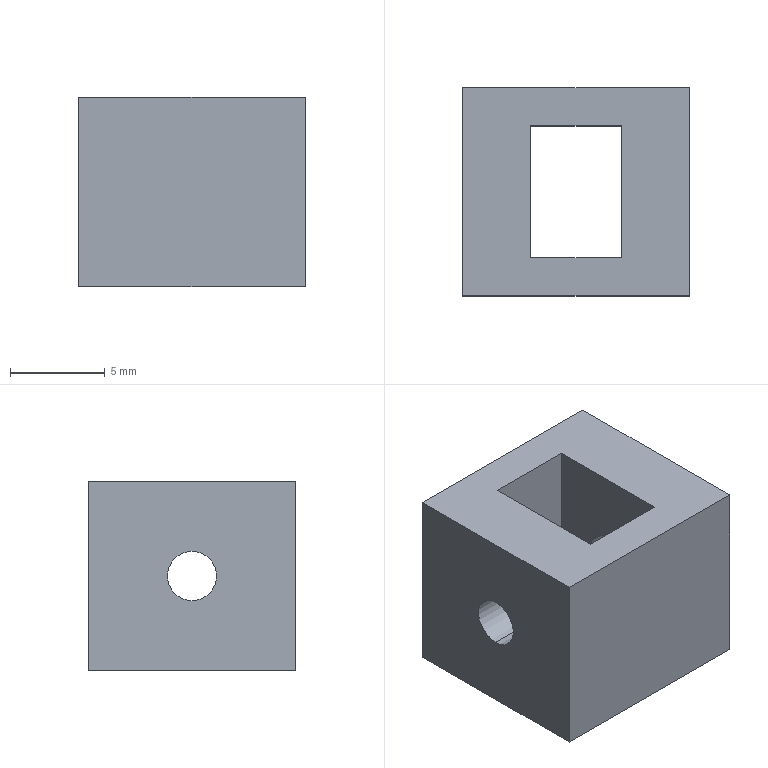Part | SolidWorks | features Extrusion 1, ICE 1 | 1 solid | 14 faces | box 11.98 x 10.98 x 10 mm | volume 942.243 mm3 | plane 10 | cylinder 4 | commonest cylinder face diameters 2.6 x4
STEP:
#1=CARTESIAN_POINT('',(-2.,3.49,6.3));
#2=VERTEX_POINT('',#1);
#3=CARTESIAN_POINT('',(-2.,3.49,3.7));
#4=VERTEX_POINT('',#3);
#5=CARTESIAN_POINT('',(-2.,3.49,5.));
#6=DIRECTION('',(1.,0.,0.));
#7=DIRECTION('',(0.,0.,-1.));
#8=AXIS2_PLACEMENT_3D('',#5,#6,#7);
#9=CIRCLE('',#8,1.3);
#10=EDGE_CURVE('',#2,#4,#9,.T.);
#11=ORIENTED_EDGE('',*,*,#10,.F.);
#12=CARTESIAN_POINT('',(1.59,3.49,6.3));
#13=VERTEX_POINT('',#12);
#14=CARTESIAN_POINT('',(-2.,3.49,6.3));
#15=DIRECTION('',(1.,0.,0.));
#16=VECTOR('',#15,1000.);
#17=LINE('',#14,#16);
#18=EDGE_CURVE('',#2,#13,#17,.T.);
#19=ORIENTED_EDGE('',*,*,#18,.T.);
#20=CARTESIAN_POINT('',(1.59,3.49,3.7));
#21=VERTEX_POINT('',#20);
#22=CARTESIAN_POINT('',(1.59,3.49,5.));
#23=DIRECTION('',(1.,0.,0.));
#24=DIRECTION('',(0.,1.,0.));
#25=AXIS2_PLACEMENT_3D('',#22,#23,#24);
#26=CIRCLE('',#25,1.3);
#27=EDGE_CURVE('',#13,#21,#26,.T.);
#28=ORIENTED_EDGE('',*,*,#27,.T.);
#29=CARTESIAN_POINT('',(-2.,3.49,3.7));
#30=DIRECTION('',(1.,0.,0.));
#31=VECTOR('',#30,1000.);
#32=LINE('',#29,#31);
#33=EDGE_CURVE('',#4,#21,#32,.T.);
#34=ORIENTED_EDGE('',*,*,#33,.F.);
#35=EDGE_LOOP('',(#11,#19,#28,#34));
#36=FACE_OUTER_BOUND('',#35,.T.);
#37=CARTESIAN_POINT('',(-2.,3.49,5.));
#38=DIRECTION('',(1.,0.,0.));
#39=DIRECTION('',(0.,0.,-1.));
#40=AXIS2_PLACEMENT_3D('',#37,#38,#39);
#41=CYLINDRICAL_SURFACE('',#40,1.3);
#42=ADVANCED_FACE('',(#36),#41,.F.);
#43=CARTESIAN_POINT('',(6.39,3.49,3.7));
#44=VERTEX_POINT('',#43);
#45=CARTESIAN_POINT('',(6.39,3.49,6.3));
#46=VERTEX_POINT('',#45);
#47=CARTESIAN_POINT('',(6.39,3.49,5.));
#48=DIRECTION('',(-1.,0.,0.));
#49=DIRECTION('',(0.,0.,1.));
#50=AXIS2_PLACEMENT_3D('',#47,#48,#49);
#51=CIRCLE('',#50,1.3);
#52=EDGE_CURVE('',#44,#46,#51,.T.);
#53=ORIENTED_EDGE('',*,*,#52,.T.);
#54=CARTESIAN_POINT('',(9.98,3.49,6.3));
#55=VERTEX_POINT('',#54);
#56=CARTESIAN_POINT('',(-2.,3.49,6.3));
#57=DIRECTION('',(1.,0.,0.));
#58=VECTOR('',#57,1000.);
#59=LINE('',#56,#58);
#60=EDGE_CURVE('',#46,#55,#59,.T.);
#61=ORIENTED_EDGE('',*,*,#60,.T.);
#62=CARTESIAN_POINT('',(9.98,3.49,3.7));
#63=VERTEX_POINT('',#62);
#64=CARTESIAN_POINT('',(9.98,3.49,5.));
#65=DIRECTION('',(1.,0.,0.));
#66=DIRECTION('',(0.,0.,-1.));
#67=AXIS2_PLACEMENT_3D('',#64,#65,#66);
#68=CIRCLE('',#67,1.3);
#69=EDGE_CURVE('',#55,#63,#68,.T.);
#70=ORIENTED_EDGE('',*,*,#69,.T.);
#71=CARTESIAN_POINT('',(-2.,3.49,3.7));
#72=DIRECTION('',(1.,0.,0.));
#73=VECTOR('',#72,1000.);
#74=LINE('',#71,#73);
#75=EDGE_CURVE('',#44,#63,#74,.T.);
#76=ORIENTED_EDGE('',*,*,#75,.F.);
#77=EDGE_LOOP('',(#53,#61,#70,#76));
#78=FACE_OUTER_BOUND('',#77,.T.);
#79=CARTESIAN_POINT('',(-2.,3.49,5.));
#80=DIRECTION('',(1.,0.,0.));
#81=DIRECTION('',(0.,0.,-1.));
#82=AXIS2_PLACEMENT_3D('',#79,#80,#81);
#83=CYLINDRICAL_SURFACE('',#82,1.3);
#84=ADVANCED_FACE('',(#78),#83,.F.);
#85=CARTESIAN_POINT('',(9.98,8.98,10.));
#86=VERTEX_POINT('',#85);
#87=CARTESIAN_POINT('',(-2.,8.98,10.));
#88=VERTEX_POINT('',#87);
#89=CARTESIAN_POINT('',(6.39,8.98,10.));
#90=DIRECTION('',(-1.,0.,0.));
#91=VECTOR('',#90,1000.);
#92=LINE('',#89,#91);
#93=EDGE_CURVE('',#86,#88,#92,.T.);
#94=ORIENTED_EDGE('',*,*,#93,.T.);
#95=CARTESIAN_POINT('',(-2.,-2.,10.));
#96=VERTEX_POINT('',#95);
#97=CARTESIAN_POINT('',(-2.,-2.,10.));
#98=DIRECTION('',(0.,-1.,0.));
#99=VECTOR('',#98,1000.);
#100=LINE('',#97,#99);
#101=EDGE_CURVE('',#88,#96,#100,.T.);
#102=ORIENTED_EDGE('',*,*,#101,.T.);
#103=CARTESIAN_POINT('',(9.98,-2.,10.));
#104=VERTEX_POINT('',#103);
#105=CARTESIAN_POINT('',(-2.,-2.,10.));
#106=DIRECTION('',(1.,0.,0.));
#107=VECTOR('',#106,1000.);
#108=LINE('',#105,#107);
#109=EDGE_CURVE('',#96,#104,#108,.T.);
#110=ORIENTED_EDGE('',*,*,#109,.T.);
#111=CARTESIAN_POINT('',(9.98,8.98,10.));
#112=DIRECTION('',(0.,1.,0.));
#113=VECTOR('',#112,1000.);
#114=LINE('',#111,#113);
#115=EDGE_CURVE('',#104,#86,#114,.T.);
#116=ORIENTED_EDGE('',*,*,#115,.T.);
#117=EDGE_LOOP('',(#94,#102,#110,#116));
#118=FACE_OUTER_BOUND('',#117,.T.);
#119=CARTESIAN_POINT('',(6.39,6.98,10.));
#120=VERTEX_POINT('',#119);
#121=CARTESIAN_POINT('',(1.59,6.98,10.));
#122=VERTEX_POINT('',#121);
#123=CARTESIAN_POINT('',(4.8,6.98,10.));
#124=DIRECTION('',(-1.,0.,0.));
#125=VECTOR('',#124,1000.);
#126=LINE('',#123,#125);
#127=EDGE_CURVE('',#120,#122,#126,.T.);
#128=ORIENTED_EDGE('',*,*,#127,.F.);
#129=CARTESIAN_POINT('',(6.39,0.,10.));
#130=VERTEX_POINT('',#129);
#131=CARTESIAN_POINT('',(6.39,6.98,10.));
#132=DIRECTION('',(0.,1.,0.));
#133=VECTOR('',#132,1000.);
#134=LINE('',#131,#133);
#135=EDGE_CURVE('',#130,#120,#134,.T.);
#136=ORIENTED_EDGE('',*,*,#135,.F.);
#137=CARTESIAN_POINT('',(1.59,0.,10.));
#138=VERTEX_POINT('',#137);
#139=CARTESIAN_POINT('',(1.59,0.,10.));
#140=DIRECTION('',(1.,0.,0.));
#141=VECTOR('',#140,1000.);
#142=LINE('',#139,#141);
#143=EDGE_CURVE('',#138,#130,#142,.T.);
#144=ORIENTED_EDGE('',*,*,#143,.F.);
#145=CARTESIAN_POINT('',(1.59,3.49,10.));
#146=DIRECTION('',(0.,-1.,0.));
#147=VECTOR('',#146,1000.);
#148=LINE('',#145,#147);
#149=EDGE_CURVE('',#122,#138,#148,.T.);
#150=ORIENTED_EDGE('',*,*,#149,.F.);
#151=EDGE_LOOP('',(#128,#136,#144,#150));
#152=FACE_BOUND('',#151,.T.);
#153=CARTESIAN_POINT('',(0.,0.,10.));
#154=DIRECTION('',(0.,0.,-1.));
#155=DIRECTION('',(-1.,0.,0.));
#156=AXIS2_PLACEMENT_3D('',#153,#154,#155);
#157=PLANE('',#156);
#158=ADVANCED_FACE('',(#118,#152),#157,.F.);
#159=CARTESIAN_POINT('',(9.98,8.98,0.));
#160=VERTEX_POINT('',#159);
#161=CARTESIAN_POINT('',(-2.,8.98,0.));
#162=VERTEX_POINT('',#161);
#163=CARTESIAN_POINT('',(-2.,8.98,0.));
#164=DIRECTION('',(-1.,0.,0.));
#165=VECTOR('',#164,1000.);
#166=LINE('',#163,#165);
#167=EDGE_CURVE('',#160,#162,#166,.T.);
#168=ORIENTED_EDGE('',*,*,#167,.F.);
#169=CARTESIAN_POINT('',(9.98,-2.,0.));
#170=VERTEX_POINT('',#169);
#171=CARTESIAN_POINT('',(9.98,8.98,0.));
#172=DIRECTION('',(0.,1.,0.));
#173=VECTOR('',#172,1000.);
#174=LINE('',#171,#173);
#175=EDGE_CURVE('',#170,#160,#174,.T.);
#176=ORIENTED_EDGE('',*,*,#175,.F.);
#177=CARTESIAN_POINT('',(-2.,-2.,0.));
#178=VERTEX_POINT('',#177);
#179=CARTESIAN_POINT('',(9.98,-2.,0.));
#180=DIRECTION('',(1.,0.,0.));
#181=VECTOR('',#180,1000.);
#182=LINE('',#179,#181);
#183=EDGE_CURVE('',#178,#170,#182,.T.);
#184=ORIENTED_EDGE('',*,*,#183,.F.);
#185=CARTESIAN_POINT('',(-2.,-2.,0.));
#186=DIRECTION('',(0.,-1.,0.));
#187=VECTOR('',#186,1000.);
#188=LINE('',#185,#187);
#189=EDGE_CURVE('',#162,#178,#188,.T.);
#190=ORIENTED_EDGE('',*,*,#189,.F.);
#191=EDGE_LOOP('',(#168,#176,#184,#190));
#192=FACE_OUTER_BOUND('',#191,.T.);
#193=CARTESIAN_POINT('',(6.39,0.,0.));
#194=VERTEX_POINT('',#193);
#195=CARTESIAN_POINT('',(6.39,6.98,0.));
#196=VERTEX_POINT('',#195);
#197=CARTESIAN_POINT('',(6.39,6.98,0.));
#198=DIRECTION('',(0.,1.,0.));
#199=VECTOR('',#198,1000.);
#200=LINE('',#197,#199);
#201=EDGE_CURVE('',#194,#196,#200,.T.);
#202=ORIENTED_EDGE('',*,*,#201,.T.);
#203=CARTESIAN_POINT('',(1.59,6.98,0.));
#204=VERTEX_POINT('',#203);
#205=CARTESIAN_POINT('',(1.59,6.98,0.));
#206=DIRECTION('',(-1.,0.,0.));
#207=VECTOR('',#206,1000.);
#208=LINE('',#205,#207);
#209=EDGE_CURVE('',#196,#204,#208,.T.);
#210=ORIENTED_EDGE('',*,*,#209,.T.);
#211=CARTESIAN_POINT('',(1.59,0.,0.));
#212=VERTEX_POINT('',#211);
#213=CARTESIAN_POINT('',(1.59,3.49,0.));
#214=DIRECTION('',(0.,-1.,0.));
#215=VECTOR('',#214,1000.);
#216=LINE('',#213,#215);
#217=EDGE_CURVE('',#204,#212,#216,.T.);
#218=ORIENTED_EDGE('',*,*,#217,.T.);
#219=CARTESIAN_POINT('',(6.39,0.,0.));
#220=DIRECTION('',(1.,0.,0.));
#221=VECTOR('',#220,1000.);
#222=LINE('',#219,#221);
#223=EDGE_CURVE('',#212,#194,#222,.T.);
#224=ORIENTED_EDGE('',*,*,#223,.T.);
#225=EDGE_LOOP('',(#202,#210,#218,#224));
#226=FACE_BOUND('',#225,.T.);
#227=CARTESIAN_POINT('',(0.,0.,0.));
#228=DIRECTION('',(0.,0.,-1.));
#229=DIRECTION('',(-1.,0.,0.));
#230=AXIS2_PLACEMENT_3D('',#227,#228,#229);
#231=PLANE('',#230);
#232=ADVANCED_FACE('',(#192,#226),#231,.T.);
#233=ORIENTED_EDGE('',*,*,#167,.T.);
#234=CARTESIAN_POINT('',(-2.,8.98,10.));
#235=DIRECTION('',(0.,0.,-1.));
#236=VECTOR('',#235,1000.);
#237=LINE('',#234,#236);
#238=EDGE_CURVE('',#88,#162,#237,.T.);
#239=ORIENTED_EDGE('',*,*,#238,.F.);
#240=ORIENTED_EDGE('',*,*,#93,.F.);
#241=CARTESIAN_POINT('',(9.98,8.98,10.));
#242=DIRECTION('',(0.,0.,-1.));
#243=VECTOR('',#242,1000.);
#244=LINE('',#241,#243);
#245=EDGE_CURVE('',#86,#160,#244,.T.);
#246=ORIENTED_EDGE('',*,*,#245,.T.);
#247=EDGE_LOOP('',(#233,#239,#240,#246));
#248=FACE_OUTER_BOUND('',#247,.T.);
#249=CARTESIAN_POINT('',(-2.,8.98,10.));
#250=DIRECTION('',(0.,-1.,0.));
#251=DIRECTION('',(0.,0.,-1.));
#252=AXIS2_PLACEMENT_3D('',#249,#250,#251);
#253=PLANE('',#252);
#254=ADVANCED_FACE('',(#248),#253,.F.);
#255=CARTESIAN_POINT('',(-2.,3.49,5.));
#256=DIRECTION('',(1.,0.,0.));
#257=DIRECTION('',(0.,0.,-1.));
#258=AXIS2_PLACEMENT_3D('',#255,#256,#257);
#259=CIRCLE('',#258,1.3);
#260=EDGE_CURVE('',#4,#2,#259,.T.);
#261=ORIENTED_EDGE('',*,*,#260,.T.);
#262=ORIENTED_EDGE('',*,*,#10,.T.);
#263=EDGE_LOOP('',(#261,#262));
#264=FACE_BOUND('',#263,.T.);
#265=ORIENTED_EDGE('',*,*,#189,.T.);
#266=CARTESIAN_POINT('',(-2.,-2.,10.));
#267=DIRECTION('',(0.,0.,-1.));
#268=VECTOR('',#267,1000.);
#269=LINE('',#266,#268);
#270=EDGE_CURVE('',#96,#178,#269,.T.);
#271=ORIENTED_EDGE('',*,*,#270,.F.);
#272=ORIENTED_EDGE('',*,*,#101,.F.);
#273=ORIENTED_EDGE('',*,*,#238,.T.);
#274=EDGE_LOOP('',(#265,#271,#272,#273));
#275=FACE_OUTER_BOUND('',#274,.T.);
#276=CARTESIAN_POINT('',(-2.,-2.,10.));
#277=DIRECTION('',(1.,0.,0.));
#278=DIRECTION('',(0.,0.,-1.));
#279=AXIS2_PLACEMENT_3D('',#276,#277,#278);
#280=PLANE('',#279);
#281=ADVANCED_FACE('',(#264,#275),#280,.F.);
#282=ORIENTED_EDGE('',*,*,#183,.T.);
#283=CARTESIAN_POINT('',(9.98,-2.,10.));
#284=DIRECTION('',(0.,0.,-1.));
#285=VECTOR('',#284,1000.);
#286=LINE('',#283,#285);
#287=EDGE_CURVE('',#104,#170,#286,.T.);
#288=ORIENTED_EDGE('',*,*,#287,.F.);
#289=ORIENTED_EDGE('',*,*,#109,.F.);
#290=ORIENTED_EDGE('',*,*,#270,.T.);
#291=EDGE_LOOP('',(#282,#288,#289,#290));
#292=FACE_OUTER_BOUND('',#291,.T.);
#293=CARTESIAN_POINT('',(9.98,-2.,10.));
#294=DIRECTION('',(0.,1.,0.));
#295=DIRECTION('',(0.,0.,1.));
#296=AXIS2_PLACEMENT_3D('',#293,#294,#295);
#297=PLANE('',#296);
#298=ADVANCED_FACE('',(#292),#297,.F.);
#299=CARTESIAN_POINT('',(9.98,3.49,5.));
#300=DIRECTION('',(1.,0.,0.));
#301=DIRECTION('',(0.,0.,-1.));
#302=AXIS2_PLACEMENT_3D('',#299,#300,#301);
#303=CIRCLE('',#302,1.3);
#304=EDGE_CURVE('',#63,#55,#303,.T.);
#305=ORIENTED_EDGE('',*,*,#304,.F.);
#306=ORIENTED_EDGE('',*,*,#69,.F.);
#307=EDGE_LOOP('',(#305,#306));
#308=FACE_BOUND('',#307,.T.);
#309=ORIENTED_EDGE('',*,*,#175,.T.);
#310=ORIENTED_EDGE('',*,*,#245,.F.);
#311=ORIENTED_EDGE('',*,*,#115,.F.);
#312=ORIENTED_EDGE('',*,*,#287,.T.);
#313=EDGE_LOOP('',(#309,#310,#311,#312));
#314=FACE_OUTER_BOUND('',#313,.T.);
#315=CARTESIAN_POINT('',(9.98,8.98,10.));
#316=DIRECTION('',(-1.,0.,0.));
#317=DIRECTION('',(0.,0.,1.));
#318=AXIS2_PLACEMENT_3D('',#315,#316,#317);
#319=PLANE('',#318);
#320=ADVANCED_FACE('',(#308,#314),#319,.F.);
#321=ORIENTED_EDGE('',*,*,#209,.F.);
#322=CARTESIAN_POINT('',(6.39,6.98,10.));
#323=DIRECTION('',(0.,0.,-1.));
#324=VECTOR('',#323,1000.);
#325=LINE('',#322,#324);
#326=EDGE_CURVE('',#120,#196,#325,.T.);
#327=ORIENTED_EDGE('',*,*,#326,.F.);
#328=ORIENTED_EDGE('',*,*,#127,.T.);
#329=CARTESIAN_POINT('',(1.59,6.98,10.));
#330=DIRECTION('',(0.,0.,-1.));
#331=VECTOR('',#330,1000.);
#332=LINE('',#329,#331);
#333=EDGE_CURVE('',#122,#204,#332,.T.);
#334=ORIENTED_EDGE('',*,*,#333,.T.);
#335=EDGE_LOOP('',(#321,#327,#328,#334));
#336=FACE_OUTER_BOUND('',#335,.T.);
#337=CARTESIAN_POINT('',(1.59,6.98,10.));
#338=DIRECTION('',(0.,-1.,0.));
#339=DIRECTION('',(0.,0.,-1.));
#340=AXIS2_PLACEMENT_3D('',#337,#338,#339);
#341=PLANE('',#340);
#342=ADVANCED_FACE('',(#336),#341,.T.);
#343=CARTESIAN_POINT('',(1.59,3.49,5.));
#344=DIRECTION('',(1.,0.,0.));
#345=DIRECTION('',(0.,1.,0.));
#346=AXIS2_PLACEMENT_3D('',#343,#344,#345);
#347=CIRCLE('',#346,1.3);
#348=EDGE_CURVE('',#21,#13,#347,.T.);
#349=ORIENTED_EDGE('',*,*,#348,.F.);
#350=ORIENTED_EDGE('',*,*,#27,.F.);
#351=EDGE_LOOP('',(#349,#350));
#352=FACE_BOUND('',#351,.T.);
#353=ORIENTED_EDGE('',*,*,#217,.F.);
#354=ORIENTED_EDGE('',*,*,#333,.F.);
#355=ORIENTED_EDGE('',*,*,#149,.T.);
#356=CARTESIAN_POINT('',(1.59,0.,10.));
#357=DIRECTION('',(0.,0.,-1.));
#358=VECTOR('',#357,1000.);
#359=LINE('',#356,#358);
#360=EDGE_CURVE('',#138,#212,#359,.T.);
#361=ORIENTED_EDGE('',*,*,#360,.T.);
#362=EDGE_LOOP('',(#353,#354,#355,#361));
#363=FACE_OUTER_BOUND('',#362,.T.);
#364=CARTESIAN_POINT('',(1.59,3.49,10.));
#365=DIRECTION('',(1.,0.,0.));
#366=DIRECTION('',(0.,1.,0.));
#367=AXIS2_PLACEMENT_3D('',#364,#365,#366);
#368=PLANE('',#367);
#369=ADVANCED_FACE('',(#352,#363),#368,.T.);
#370=ORIENTED_EDGE('',*,*,#223,.F.);
#371=ORIENTED_EDGE('',*,*,#360,.F.);
#372=ORIENTED_EDGE('',*,*,#143,.T.);
#373=CARTESIAN_POINT('',(6.39,0.,10.));
#374=DIRECTION('',(0.,0.,-1.));
#375=VECTOR('',#374,1000.);
#376=LINE('',#373,#375);
#377=EDGE_CURVE('',#130,#194,#376,.T.);
#378=ORIENTED_EDGE('',*,*,#377,.T.);
#379=EDGE_LOOP('',(#370,#371,#372,#378));
#380=FACE_OUTER_BOUND('',#379,.T.);
#381=CARTESIAN_POINT('',(6.39,0.,10.));
#382=DIRECTION('',(0.,1.,0.));
#383=DIRECTION('',(0.,0.,1.));
#384=AXIS2_PLACEMENT_3D('',#381,#382,#383);
#385=PLANE('',#384);
#386=ADVANCED_FACE('',(#380),#385,.T.);
#387=ORIENTED_EDGE('',*,*,#52,.F.);
#388=CARTESIAN_POINT('',(6.39,3.49,5.));
#389=DIRECTION('',(-1.,0.,0.));
#390=DIRECTION('',(0.,0.,1.));
#391=AXIS2_PLACEMENT_3D('',#388,#389,#390);
#392=CIRCLE('',#391,1.3);
#393=EDGE_CURVE('',#46,#44,#392,.T.);
#394=ORIENTED_EDGE('',*,*,#393,.F.);
#395=EDGE_LOOP('',(#387,#394));
#396=FACE_BOUND('',#395,.T.);
#397=ORIENTED_EDGE('',*,*,#201,.F.);
#398=ORIENTED_EDGE('',*,*,#377,.F.);
#399=ORIENTED_EDGE('',*,*,#135,.T.);
#400=ORIENTED_EDGE('',*,*,#326,.T.);
#401=EDGE_LOOP('',(#397,#398,#399,#400));
#402=FACE_OUTER_BOUND('',#401,.T.);
#403=CARTESIAN_POINT('',(6.39,6.98,10.));
#404=DIRECTION('',(-1.,0.,0.));
#405=DIRECTION('',(0.,0.,1.));
#406=AXIS2_PLACEMENT_3D('',#403,#404,#405);
#407=PLANE('',#406);
#408=ADVANCED_FACE('',(#396,#402),#407,.T.);
#409=ORIENTED_EDGE('',*,*,#60,.F.);
#410=ORIENTED_EDGE('',*,*,#393,.T.);
#411=ORIENTED_EDGE('',*,*,#75,.T.);
#412=ORIENTED_EDGE('',*,*,#304,.T.);
#413=EDGE_LOOP('',(#409,#410,#411,#412));
#414=FACE_OUTER_BOUND('',#413,.T.);
#415=CARTESIAN_POINT('',(-2.,3.49,5.));
#416=DIRECTION('',(1.,0.,0.));
#417=DIRECTION('',(0.,0.,-1.));
#418=AXIS2_PLACEMENT_3D('',#415,#416,#417);
#419=CYLINDRICAL_SURFACE('',#418,1.3);
#420=ADVANCED_FACE('',(#414),#419,.F.);
#421=ORIENTED_EDGE('',*,*,#18,.F.);
#422=ORIENTED_EDGE('',*,*,#260,.F.);
#423=ORIENTED_EDGE('',*,*,#33,.T.);
#424=ORIENTED_EDGE('',*,*,#348,.T.);
#425=EDGE_LOOP('',(#421,#422,#423,#424));
#426=FACE_OUTER_BOUND('',#425,.T.);
#427=CARTESIAN_POINT('',(-2.,3.49,5.));
#428=DIRECTION('',(1.,0.,0.));
#429=DIRECTION('',(0.,0.,-1.));
#430=AXIS2_PLACEMENT_3D('',#427,#428,#429);
#431=CYLINDRICAL_SURFACE('',#430,1.3);
#432=ADVANCED_FACE('',(#426),#431,.F.);
#433=CLOSED_SHELL('',(#42,#84,#158,#232,#254,#281,#298,#320,#342,#369,#386,#408,#420,#432));
#434=MANIFOLD_SOLID_BREP('',#433);
#435=CARTESIAN_POINT('',(0.,0.,0.));
#436=DIRECTION('',(0.,0.,1.));
#437=DIRECTION('',(1.,0.,0.));
#438=AXIS2_PLACEMENT_3D('',#435,#436,#437);
#439=(LENGTH_UNIT()NAMED_UNIT(*)SI_UNIT(.MILLI.,.METRE.));
#440=UNCERTAINTY_MEASURE_WITH_UNIT(LENGTH_MEASURE(0.00001),#439,'','');
#441=(NAMED_UNIT(*)PLANE_ANGLE_UNIT()SI_UNIT($,.RADIAN.));
#442=(NAMED_UNIT(*)SI_UNIT($,.STERADIAN.)SOLID_ANGLE_UNIT());
#443=(GEOMETRIC_REPRESENTATION_CONTEXT(3)GLOBAL_UNCERTAINTY_ASSIGNED_CONTEXT((#440))GLOBAL_UNIT_ASSIGNED_CONTEXT((#439,#441,#442))REPRESENTATION_CONTEXT('',''));
#444=ADVANCED_BREP_SHAPE_REPRESENTATION('',(#434,#438),#443);